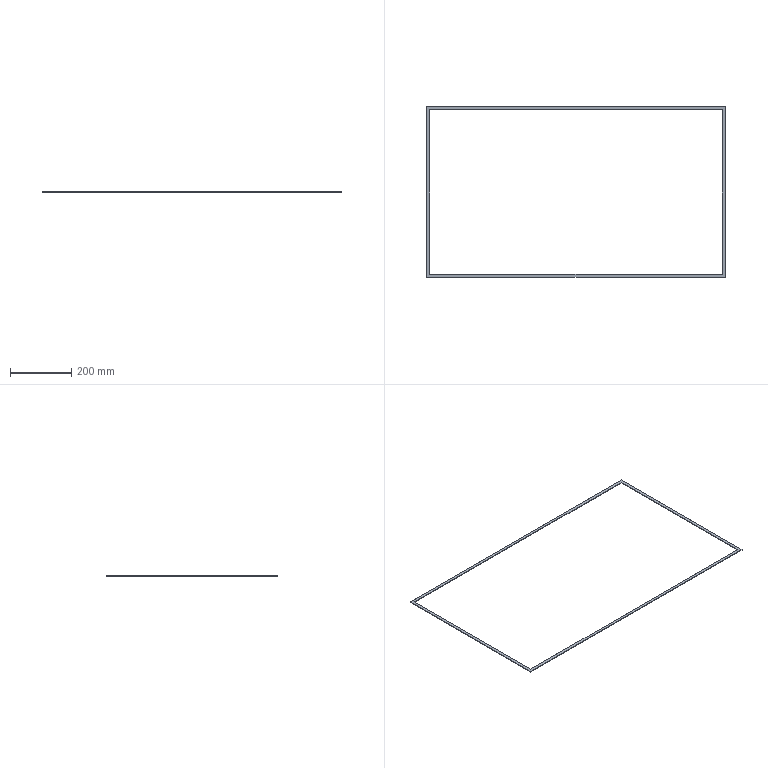Part | SolidWorks | features Extrusion 1, Fillet 1 | 1 solid | 14 faces | box 974.6 x 557 x 2 mm | volume 60464 mm3 | plane 10 | cylinder 4 | commonest cylinder face diameters 0.4 x4
STEP:
#1=CARTESIAN_POINT('',(-487.3,278.5,2.));
#2=VERTEX_POINT('',#1);
#3=CARTESIAN_POINT('',(-487.3,-278.5,2.));
#4=VERTEX_POINT('',#3);
#5=CARTESIAN_POINT('',(-487.3,278.5,2.));
#6=DIRECTION('',(0.,-1.,0.));
#7=VECTOR('',#6,1000.);
#8=LINE('',#5,#7);
#9=EDGE_CURVE('',#2,#4,#8,.T.);
#10=ORIENTED_EDGE('',*,*,#9,.T.);
#11=CARTESIAN_POINT('',(487.3,-278.5,2.));
#12=VERTEX_POINT('',#11);
#13=CARTESIAN_POINT('',(-487.3,-278.5,2.));
#14=DIRECTION('',(1.,0.,0.));
#15=VECTOR('',#14,1000.);
#16=LINE('',#13,#15);
#17=EDGE_CURVE('',#4,#12,#16,.T.);
#18=ORIENTED_EDGE('',*,*,#17,.T.);
#19=CARTESIAN_POINT('',(487.3,278.5,2.));
#20=VERTEX_POINT('',#19);
#21=CARTESIAN_POINT('',(487.3,278.5,2.));
#22=DIRECTION('',(0.,1.,0.));
#23=VECTOR('',#22,1000.);
#24=LINE('',#21,#23);
#25=EDGE_CURVE('',#12,#20,#24,.T.);
#26=ORIENTED_EDGE('',*,*,#25,.T.);
#27=CARTESIAN_POINT('',(-487.3,278.5,2.));
#28=DIRECTION('',(-1.,0.,0.));
#29=VECTOR('',#28,1000.);
#30=LINE('',#27,#29);
#31=EDGE_CURVE('',#20,#2,#30,.T.);
#32=ORIENTED_EDGE('',*,*,#31,.T.);
#33=EDGE_LOOP('',(#10,#18,#26,#32));
#34=FACE_OUTER_BOUND('',#33,.T.);
#35=CARTESIAN_POINT('',(477.1,268.5,2.));
#36=VERTEX_POINT('',#35);
#37=CARTESIAN_POINT('',(-477.1,268.5,2.));
#38=VERTEX_POINT('',#37);
#39=CARTESIAN_POINT('',(-477.3,268.5,2.));
#40=DIRECTION('',(-1.,0.,0.));
#41=VECTOR('',#40,1000.);
#42=LINE('',#39,#41);
#43=EDGE_CURVE('',#36,#38,#42,.T.);
#44=ORIENTED_EDGE('',*,*,#43,.F.);
#45=CARTESIAN_POINT('',(477.3,268.3,2.));
#46=VERTEX_POINT('',#45);
#47=CARTESIAN_POINT('',(477.1,268.3,2.));
#48=DIRECTION('',(0.,0.,-1.));
#49=DIRECTION('',(1.,0.,0.));
#50=AXIS2_PLACEMENT_3D('',#47,#48,#49);
#51=CIRCLE('',#50,0.2);
#52=EDGE_CURVE('',#36,#46,#51,.T.);
#53=ORIENTED_EDGE('',*,*,#52,.T.);
#54=CARTESIAN_POINT('',(477.3,-268.3,2.));
#55=VERTEX_POINT('',#54);
#56=CARTESIAN_POINT('',(477.3,268.5,2.));
#57=DIRECTION('',(0.,1.,0.));
#58=VECTOR('',#57,1000.);
#59=LINE('',#56,#58);
#60=EDGE_CURVE('',#55,#46,#59,.T.);
#61=ORIENTED_EDGE('',*,*,#60,.F.);
#62=CARTESIAN_POINT('',(477.1,-268.5,2.));
#63=VERTEX_POINT('',#62);
#64=CARTESIAN_POINT('',(477.1,-268.3,2.));
#65=DIRECTION('',(0.,0.,-1.));
#66=DIRECTION('',(1.,0.,0.));
#67=AXIS2_PLACEMENT_3D('',#64,#65,#66);
#68=CIRCLE('',#67,0.2);
#69=EDGE_CURVE('',#55,#63,#68,.T.);
#70=ORIENTED_EDGE('',*,*,#69,.T.);
#71=CARTESIAN_POINT('',(-477.1,-268.5,2.));
#72=VERTEX_POINT('',#71);
#73=CARTESIAN_POINT('',(-477.3,-268.5,2.));
#74=DIRECTION('',(1.,0.,0.));
#75=VECTOR('',#74,1000.);
#76=LINE('',#73,#75);
#77=EDGE_CURVE('',#72,#63,#76,.T.);
#78=ORIENTED_EDGE('',*,*,#77,.F.);
#79=CARTESIAN_POINT('',(-477.3,-268.3,2.));
#80=VERTEX_POINT('',#79);
#81=CARTESIAN_POINT('',(-477.1,-268.3,2.));
#82=DIRECTION('',(0.,0.,-1.));
#83=DIRECTION('',(1.,0.,0.));
#84=AXIS2_PLACEMENT_3D('',#81,#82,#83);
#85=CIRCLE('',#84,0.2);
#86=EDGE_CURVE('',#72,#80,#85,.T.);
#87=ORIENTED_EDGE('',*,*,#86,.T.);
#88=CARTESIAN_POINT('',(-477.3,268.3,2.));
#89=VERTEX_POINT('',#88);
#90=CARTESIAN_POINT('',(-477.3,268.5,2.));
#91=DIRECTION('',(0.,-1.,0.));
#92=VECTOR('',#91,1000.);
#93=LINE('',#90,#92);
#94=EDGE_CURVE('',#89,#80,#93,.T.);
#95=ORIENTED_EDGE('',*,*,#94,.F.);
#96=CARTESIAN_POINT('',(-477.1,268.3,2.));
#97=DIRECTION('',(0.,0.,-1.));
#98=DIRECTION('',(1.,0.,0.));
#99=AXIS2_PLACEMENT_3D('',#96,#97,#98);
#100=CIRCLE('',#99,0.2);
#101=EDGE_CURVE('',#89,#38,#100,.T.);
#102=ORIENTED_EDGE('',*,*,#101,.T.);
#103=EDGE_LOOP('',(#44,#53,#61,#70,#78,#87,#95,#102));
#104=FACE_BOUND('',#103,.T.);
#105=CARTESIAN_POINT('',(0.,0.,2.));
#106=DIRECTION('',(0.,0.,1.));
#107=DIRECTION('',(1.,0.,0.));
#108=AXIS2_PLACEMENT_3D('',#105,#106,#107);
#109=PLANE('',#108);
#110=ADVANCED_FACE('',(#34,#104),#109,.T.);
#111=CARTESIAN_POINT('',(-487.3,278.5,0.));
#112=VERTEX_POINT('',#111);
#113=CARTESIAN_POINT('',(-487.3,-278.5,0.));
#114=VERTEX_POINT('',#113);
#115=CARTESIAN_POINT('',(-487.3,278.5,0.));
#116=DIRECTION('',(0.,-1.,0.));
#117=VECTOR('',#116,1000.);
#118=LINE('',#115,#117);
#119=EDGE_CURVE('',#112,#114,#118,.T.);
#120=ORIENTED_EDGE('',*,*,#119,.F.);
#121=CARTESIAN_POINT('',(487.3,278.5,0.));
#122=VERTEX_POINT('',#121);
#123=CARTESIAN_POINT('',(-487.3,278.5,0.));
#124=DIRECTION('',(-1.,0.,0.));
#125=VECTOR('',#124,1000.);
#126=LINE('',#123,#125);
#127=EDGE_CURVE('',#122,#112,#126,.T.);
#128=ORIENTED_EDGE('',*,*,#127,.F.);
#129=CARTESIAN_POINT('',(487.3,-278.5,0.));
#130=VERTEX_POINT('',#129);
#131=CARTESIAN_POINT('',(487.3,278.5,0.));
#132=DIRECTION('',(0.,1.,0.));
#133=VECTOR('',#132,1000.);
#134=LINE('',#131,#133);
#135=EDGE_CURVE('',#130,#122,#134,.T.);
#136=ORIENTED_EDGE('',*,*,#135,.F.);
#137=CARTESIAN_POINT('',(-487.3,-278.5,0.));
#138=DIRECTION('',(1.,0.,0.));
#139=VECTOR('',#138,1000.);
#140=LINE('',#137,#139);
#141=EDGE_CURVE('',#114,#130,#140,.T.);
#142=ORIENTED_EDGE('',*,*,#141,.F.);
#143=EDGE_LOOP('',(#120,#128,#136,#142));
#144=FACE_OUTER_BOUND('',#143,.T.);
#145=CARTESIAN_POINT('',(-477.1,-268.5,0.));
#146=VERTEX_POINT('',#145);
#147=CARTESIAN_POINT('',(477.1,-268.5,0.));
#148=VERTEX_POINT('',#147);
#149=CARTESIAN_POINT('',(-477.3,-268.5,0.));
#150=DIRECTION('',(1.,0.,0.));
#151=VECTOR('',#150,1000.);
#152=LINE('',#149,#151);
#153=EDGE_CURVE('',#146,#148,#152,.T.);
#154=ORIENTED_EDGE('',*,*,#153,.T.);
#155=CARTESIAN_POINT('',(477.3,-268.3,0.));
#156=VERTEX_POINT('',#155);
#157=CARTESIAN_POINT('',(477.1,-268.3,0.));
#158=DIRECTION('',(0.,0.,1.));
#159=DIRECTION('',(1.,0.,0.));
#160=AXIS2_PLACEMENT_3D('',#157,#158,#159);
#161=CIRCLE('',#160,0.2);
#162=EDGE_CURVE('',#148,#156,#161,.T.);
#163=ORIENTED_EDGE('',*,*,#162,.T.);
#164=CARTESIAN_POINT('',(477.3,268.3,0.));
#165=VERTEX_POINT('',#164);
#166=CARTESIAN_POINT('',(477.3,268.5,0.));
#167=DIRECTION('',(0.,1.,0.));
#168=VECTOR('',#167,1000.);
#169=LINE('',#166,#168);
#170=EDGE_CURVE('',#156,#165,#169,.T.);
#171=ORIENTED_EDGE('',*,*,#170,.T.);
#172=CARTESIAN_POINT('',(477.1,268.5,0.));
#173=VERTEX_POINT('',#172);
#174=CARTESIAN_POINT('',(477.1,268.3,0.));
#175=DIRECTION('',(0.,0.,1.));
#176=DIRECTION('',(1.,0.,0.));
#177=AXIS2_PLACEMENT_3D('',#174,#175,#176);
#178=CIRCLE('',#177,0.2);
#179=EDGE_CURVE('',#165,#173,#178,.T.);
#180=ORIENTED_EDGE('',*,*,#179,.T.);
#181=CARTESIAN_POINT('',(-477.1,268.5,0.));
#182=VERTEX_POINT('',#181);
#183=CARTESIAN_POINT('',(-477.3,268.5,0.));
#184=DIRECTION('',(-1.,0.,0.));
#185=VECTOR('',#184,1000.);
#186=LINE('',#183,#185);
#187=EDGE_CURVE('',#173,#182,#186,.T.);
#188=ORIENTED_EDGE('',*,*,#187,.T.);
#189=CARTESIAN_POINT('',(-477.3,268.3,0.));
#190=VERTEX_POINT('',#189);
#191=CARTESIAN_POINT('',(-477.1,268.3,0.));
#192=DIRECTION('',(0.,0.,1.));
#193=DIRECTION('',(1.,0.,0.));
#194=AXIS2_PLACEMENT_3D('',#191,#192,#193);
#195=CIRCLE('',#194,0.2);
#196=EDGE_CURVE('',#182,#190,#195,.T.);
#197=ORIENTED_EDGE('',*,*,#196,.T.);
#198=CARTESIAN_POINT('',(-477.3,-268.3,0.));
#199=VERTEX_POINT('',#198);
#200=CARTESIAN_POINT('',(-477.3,268.5,0.));
#201=DIRECTION('',(0.,-1.,0.));
#202=VECTOR('',#201,1000.);
#203=LINE('',#200,#202);
#204=EDGE_CURVE('',#190,#199,#203,.T.);
#205=ORIENTED_EDGE('',*,*,#204,.T.);
#206=CARTESIAN_POINT('',(-477.1,-268.3,0.));
#207=DIRECTION('',(0.,0.,1.));
#208=DIRECTION('',(1.,0.,0.));
#209=AXIS2_PLACEMENT_3D('',#206,#207,#208);
#210=CIRCLE('',#209,0.2);
#211=EDGE_CURVE('',#199,#146,#210,.T.);
#212=ORIENTED_EDGE('',*,*,#211,.T.);
#213=EDGE_LOOP('',(#154,#163,#171,#180,#188,#197,#205,#212));
#214=FACE_BOUND('',#213,.T.);
#215=CARTESIAN_POINT('',(0.,0.,0.));
#216=DIRECTION('',(0.,0.,1.));
#217=DIRECTION('',(1.,0.,0.));
#218=AXIS2_PLACEMENT_3D('',#215,#216,#217);
#219=PLANE('',#218);
#220=ADVANCED_FACE('',(#144,#214),#219,.F.);
#221=ORIENTED_EDGE('',*,*,#119,.T.);
#222=CARTESIAN_POINT('',(-487.3,-278.5,2.));
#223=DIRECTION('',(0.,0.,-1.));
#224=VECTOR('',#223,1000.);
#225=LINE('',#222,#224);
#226=EDGE_CURVE('',#4,#114,#225,.T.);
#227=ORIENTED_EDGE('',*,*,#226,.F.);
#228=ORIENTED_EDGE('',*,*,#9,.F.);
#229=CARTESIAN_POINT('',(-487.3,278.5,2.));
#230=DIRECTION('',(0.,0.,-1.));
#231=VECTOR('',#230,1000.);
#232=LINE('',#229,#231);
#233=EDGE_CURVE('',#2,#112,#232,.T.);
#234=ORIENTED_EDGE('',*,*,#233,.T.);
#235=EDGE_LOOP('',(#221,#227,#228,#234));
#236=FACE_OUTER_BOUND('',#235,.T.);
#237=CARTESIAN_POINT('',(-487.3,278.5,2.));
#238=DIRECTION('',(1.,0.,0.));
#239=DIRECTION('',(0.,1.,0.));
#240=AXIS2_PLACEMENT_3D('',#237,#238,#239);
#241=PLANE('',#240);
#242=ADVANCED_FACE('',(#236),#241,.F.);
#243=ORIENTED_EDGE('',*,*,#141,.T.);
#244=CARTESIAN_POINT('',(487.3,-278.5,2.));
#245=DIRECTION('',(0.,0.,-1.));
#246=VECTOR('',#245,1000.);
#247=LINE('',#244,#246);
#248=EDGE_CURVE('',#12,#130,#247,.T.);
#249=ORIENTED_EDGE('',*,*,#248,.F.);
#250=ORIENTED_EDGE('',*,*,#17,.F.);
#251=ORIENTED_EDGE('',*,*,#226,.T.);
#252=EDGE_LOOP('',(#243,#249,#250,#251));
#253=FACE_OUTER_BOUND('',#252,.T.);
#254=CARTESIAN_POINT('',(-487.3,-278.5,2.));
#255=DIRECTION('',(0.,1.,0.));
#256=DIRECTION('',(0.,0.,1.));
#257=AXIS2_PLACEMENT_3D('',#254,#255,#256);
#258=PLANE('',#257);
#259=ADVANCED_FACE('',(#253),#258,.F.);
#260=ORIENTED_EDGE('',*,*,#135,.T.);
#261=CARTESIAN_POINT('',(487.3,278.5,2.));
#262=DIRECTION('',(0.,0.,-1.));
#263=VECTOR('',#262,1000.);
#264=LINE('',#261,#263);
#265=EDGE_CURVE('',#20,#122,#264,.T.);
#266=ORIENTED_EDGE('',*,*,#265,.F.);
#267=ORIENTED_EDGE('',*,*,#25,.F.);
#268=ORIENTED_EDGE('',*,*,#248,.T.);
#269=EDGE_LOOP('',(#260,#266,#267,#268));
#270=FACE_OUTER_BOUND('',#269,.T.);
#271=CARTESIAN_POINT('',(487.3,278.5,2.));
#272=DIRECTION('',(-1.,0.,0.));
#273=DIRECTION('',(0.,-1.,0.));
#274=AXIS2_PLACEMENT_3D('',#271,#272,#273);
#275=PLANE('',#274);
#276=ADVANCED_FACE('',(#270),#275,.F.);
#277=ORIENTED_EDGE('',*,*,#127,.T.);
#278=ORIENTED_EDGE('',*,*,#233,.F.);
#279=ORIENTED_EDGE('',*,*,#31,.F.);
#280=ORIENTED_EDGE('',*,*,#265,.T.);
#281=EDGE_LOOP('',(#277,#278,#279,#280));
#282=FACE_OUTER_BOUND('',#281,.T.);
#283=CARTESIAN_POINT('',(-487.3,278.5,2.));
#284=DIRECTION('',(0.,-1.,0.));
#285=DIRECTION('',(0.,0.,-1.));
#286=AXIS2_PLACEMENT_3D('',#283,#284,#285);
#287=PLANE('',#286);
#288=ADVANCED_FACE('',(#282),#287,.F.);
#289=ORIENTED_EDGE('',*,*,#60,.T.);
#290=CARTESIAN_POINT('',(477.3,268.3,0.));
#291=DIRECTION('',(0.,0.,-1.));
#292=VECTOR('',#291,1000.);
#293=LINE('',#290,#292);
#294=EDGE_CURVE('',#46,#165,#293,.T.);
#295=ORIENTED_EDGE('',*,*,#294,.T.);
#296=ORIENTED_EDGE('',*,*,#170,.F.);
#297=CARTESIAN_POINT('',(477.3,-268.3,2.));
#298=DIRECTION('',(0.,0.,1.));
#299=VECTOR('',#298,1000.);
#300=LINE('',#297,#299);
#301=EDGE_CURVE('',#156,#55,#300,.T.);
#302=ORIENTED_EDGE('',*,*,#301,.T.);
#303=EDGE_LOOP('',(#289,#295,#296,#302));
#304=FACE_OUTER_BOUND('',#303,.T.);
#305=CARTESIAN_POINT('',(477.3,268.5,2.));
#306=DIRECTION('',(-1.,0.,0.));
#307=DIRECTION('',(0.,-1.,0.));
#308=AXIS2_PLACEMENT_3D('',#305,#306,#307);
#309=PLANE('',#308);
#310=ADVANCED_FACE('',(#304),#309,.T.);
#311=ORIENTED_EDGE('',*,*,#43,.T.);
#312=CARTESIAN_POINT('',(-477.1,268.5,0.));
#313=DIRECTION('',(0.,0.,-1.));
#314=VECTOR('',#313,1000.);
#315=LINE('',#312,#314);
#316=EDGE_CURVE('',#38,#182,#315,.T.);
#317=ORIENTED_EDGE('',*,*,#316,.T.);
#318=ORIENTED_EDGE('',*,*,#187,.F.);
#319=CARTESIAN_POINT('',(477.1,268.5,2.));
#320=DIRECTION('',(0.,0.,1.));
#321=VECTOR('',#320,1000.);
#322=LINE('',#319,#321);
#323=EDGE_CURVE('',#173,#36,#322,.T.);
#324=ORIENTED_EDGE('',*,*,#323,.T.);
#325=EDGE_LOOP('',(#311,#317,#318,#324));
#326=FACE_OUTER_BOUND('',#325,.T.);
#327=CARTESIAN_POINT('',(-477.3,268.5,2.));
#328=DIRECTION('',(0.,-1.,0.));
#329=DIRECTION('',(0.,0.,-1.));
#330=AXIS2_PLACEMENT_3D('',#327,#328,#329);
#331=PLANE('',#330);
#332=ADVANCED_FACE('',(#326),#331,.T.);
#333=ORIENTED_EDGE('',*,*,#94,.T.);
#334=CARTESIAN_POINT('',(-477.3,-268.3,0.));
#335=DIRECTION('',(0.,0.,-1.));
#336=VECTOR('',#335,1000.);
#337=LINE('',#334,#336);
#338=EDGE_CURVE('',#80,#199,#337,.T.);
#339=ORIENTED_EDGE('',*,*,#338,.T.);
#340=ORIENTED_EDGE('',*,*,#204,.F.);
#341=CARTESIAN_POINT('',(-477.3,268.3,2.));
#342=DIRECTION('',(0.,0.,1.));
#343=VECTOR('',#342,1000.);
#344=LINE('',#341,#343);
#345=EDGE_CURVE('',#190,#89,#344,.T.);
#346=ORIENTED_EDGE('',*,*,#345,.T.);
#347=EDGE_LOOP('',(#333,#339,#340,#346));
#348=FACE_OUTER_BOUND('',#347,.T.);
#349=CARTESIAN_POINT('',(-477.3,268.5,2.));
#350=DIRECTION('',(1.,0.,0.));
#351=DIRECTION('',(0.,1.,0.));
#352=AXIS2_PLACEMENT_3D('',#349,#350,#351);
#353=PLANE('',#352);
#354=ADVANCED_FACE('',(#348),#353,.T.);
#355=ORIENTED_EDGE('',*,*,#153,.F.);
#356=CARTESIAN_POINT('',(-477.1,-268.5,2.));
#357=DIRECTION('',(0.,0.,1.));
#358=VECTOR('',#357,1000.);
#359=LINE('',#356,#358);
#360=EDGE_CURVE('',#146,#72,#359,.T.);
#361=ORIENTED_EDGE('',*,*,#360,.T.);
#362=ORIENTED_EDGE('',*,*,#77,.T.);
#363=CARTESIAN_POINT('',(477.1,-268.5,0.));
#364=DIRECTION('',(0.,0.,-1.));
#365=VECTOR('',#364,1000.);
#366=LINE('',#363,#365);
#367=EDGE_CURVE('',#63,#148,#366,.T.);
#368=ORIENTED_EDGE('',*,*,#367,.T.);
#369=EDGE_LOOP('',(#355,#361,#362,#368));
#370=FACE_OUTER_BOUND('',#369,.T.);
#371=CARTESIAN_POINT('',(-477.3,-268.5,2.));
#372=DIRECTION('',(0.,1.,0.));
#373=DIRECTION('',(0.,0.,1.));
#374=AXIS2_PLACEMENT_3D('',#371,#372,#373);
#375=PLANE('',#374);
#376=ADVANCED_FACE('',(#370),#375,.T.);
#377=ORIENTED_EDGE('',*,*,#86,.F.);
#378=ORIENTED_EDGE('',*,*,#360,.F.);
#379=ORIENTED_EDGE('',*,*,#211,.F.);
#380=ORIENTED_EDGE('',*,*,#338,.F.);
#381=EDGE_LOOP('',(#377,#378,#379,#380));
#382=FACE_OUTER_BOUND('',#381,.T.);
#383=CARTESIAN_POINT('',(-477.1,-268.3,2.));
#384=DIRECTION('',(0.,0.,1.));
#385=DIRECTION('',(1.,0.,0.));
#386=AXIS2_PLACEMENT_3D('',#383,#384,#385);
#387=CYLINDRICAL_SURFACE('',#386,0.2);
#388=ADVANCED_FACE('',(#382),#387,.F.);
#389=ORIENTED_EDGE('',*,*,#101,.F.);
#390=ORIENTED_EDGE('',*,*,#345,.F.);
#391=ORIENTED_EDGE('',*,*,#196,.F.);
#392=ORIENTED_EDGE('',*,*,#316,.F.);
#393=EDGE_LOOP('',(#389,#390,#391,#392));
#394=FACE_OUTER_BOUND('',#393,.T.);
#395=CARTESIAN_POINT('',(-477.1,268.3,2.));
#396=DIRECTION('',(0.,0.,1.));
#397=DIRECTION('',(1.,0.,0.));
#398=AXIS2_PLACEMENT_3D('',#395,#396,#397);
#399=CYLINDRICAL_SURFACE('',#398,0.2);
#400=ADVANCED_FACE('',(#394),#399,.F.);
#401=ORIENTED_EDGE('',*,*,#52,.F.);
#402=ORIENTED_EDGE('',*,*,#323,.F.);
#403=ORIENTED_EDGE('',*,*,#179,.F.);
#404=ORIENTED_EDGE('',*,*,#294,.F.);
#405=EDGE_LOOP('',(#401,#402,#403,#404));
#406=FACE_OUTER_BOUND('',#405,.T.);
#407=CARTESIAN_POINT('',(477.1,268.3,2.));
#408=DIRECTION('',(0.,0.,1.));
#409=DIRECTION('',(1.,0.,0.));
#410=AXIS2_PLACEMENT_3D('',#407,#408,#409);
#411=CYLINDRICAL_SURFACE('',#410,0.2);
#412=ADVANCED_FACE('',(#406),#411,.F.);
#413=ORIENTED_EDGE('',*,*,#69,.F.);
#414=ORIENTED_EDGE('',*,*,#301,.F.);
#415=ORIENTED_EDGE('',*,*,#162,.F.);
#416=ORIENTED_EDGE('',*,*,#367,.F.);
#417=EDGE_LOOP('',(#413,#414,#415,#416));
#418=FACE_OUTER_BOUND('',#417,.T.);
#419=CARTESIAN_POINT('',(477.1,-268.3,2.));
#420=DIRECTION('',(0.,0.,1.));
#421=DIRECTION('',(1.,0.,0.));
#422=AXIS2_PLACEMENT_3D('',#419,#420,#421);
#423=CYLINDRICAL_SURFACE('',#422,0.2);
#424=ADVANCED_FACE('',(#418),#423,.F.);
#425=CLOSED_SHELL('',(#110,#220,#242,#259,#276,#288,#310,#332,#354,#376,#388,#400,#412,#424));
#426=MANIFOLD_SOLID_BREP('',#425);
#427=CARTESIAN_POINT('',(0.,0.,0.));
#428=DIRECTION('',(0.,0.,1.));
#429=DIRECTION('',(1.,0.,0.));
#430=AXIS2_PLACEMENT_3D('',#427,#428,#429);
#431=(LENGTH_UNIT()NAMED_UNIT(*)SI_UNIT(.MILLI.,.METRE.));
#432=UNCERTAINTY_MEASURE_WITH_UNIT(LENGTH_MEASURE(0.00001),#431,'','');
#433=(NAMED_UNIT(*)PLANE_ANGLE_UNIT()SI_UNIT($,.RADIAN.));
#434=(NAMED_UNIT(*)SI_UNIT($,.STERADIAN.)SOLID_ANGLE_UNIT());
#435=(GEOMETRIC_REPRESENTATION_CONTEXT(3)GLOBAL_UNCERTAINTY_ASSIGNED_CONTEXT((#432))GLOBAL_UNIT_ASSIGNED_CONTEXT((#431,#433,#434))REPRESENTATION_CONTEXT('',''));
#436=ADVANCED_BREP_SHAPE_REPRESENTATION('',(#426,#430),#435);